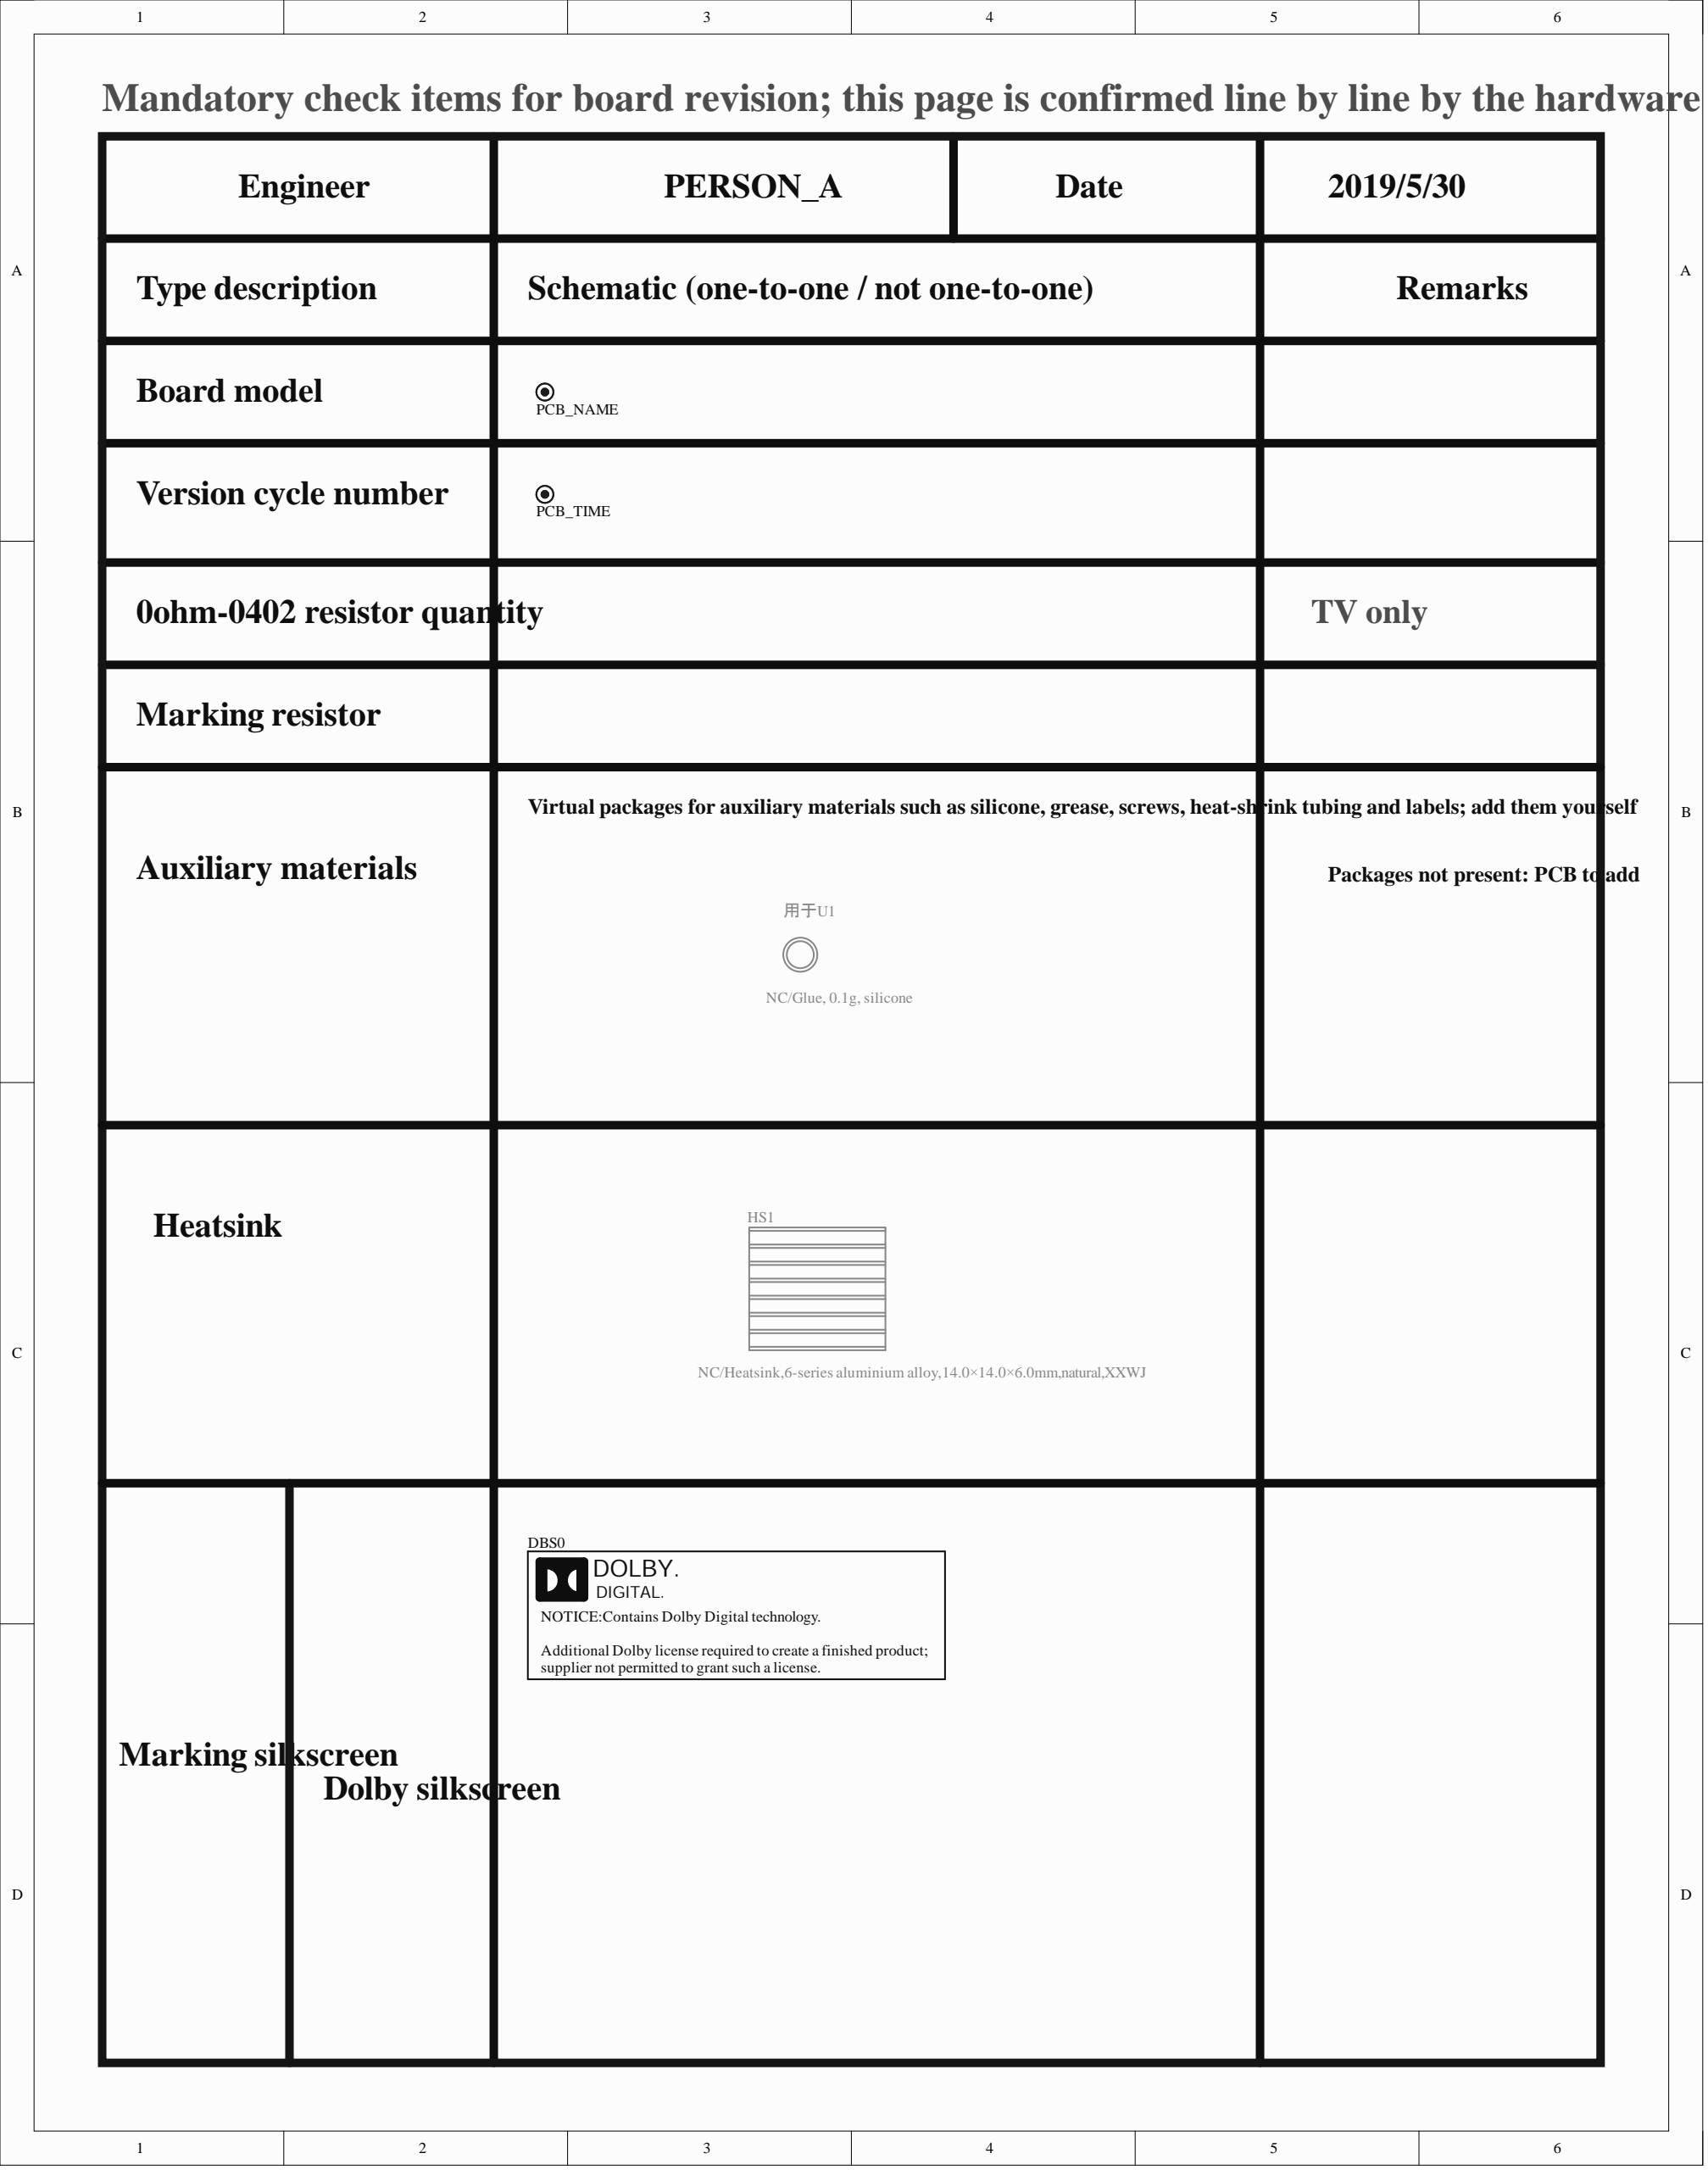Circuit board | Altium Designer | 578 parts | 300 nets | one sheet of the schematic
Parts on this sheet (reference | value | footprint):
DBS0 | DOLBY | DOLBY-SILK
HS1 | NC/Heatsink,6-series aluminium alloy,14.0×14.0×6.0mm,natural,XXWJ | HS(14*14*6)
用于U1 | NC/Glue, 0.1g, silicone | Heat-Shrinkable Tube
Nets of these parts (net: part-pin ...):